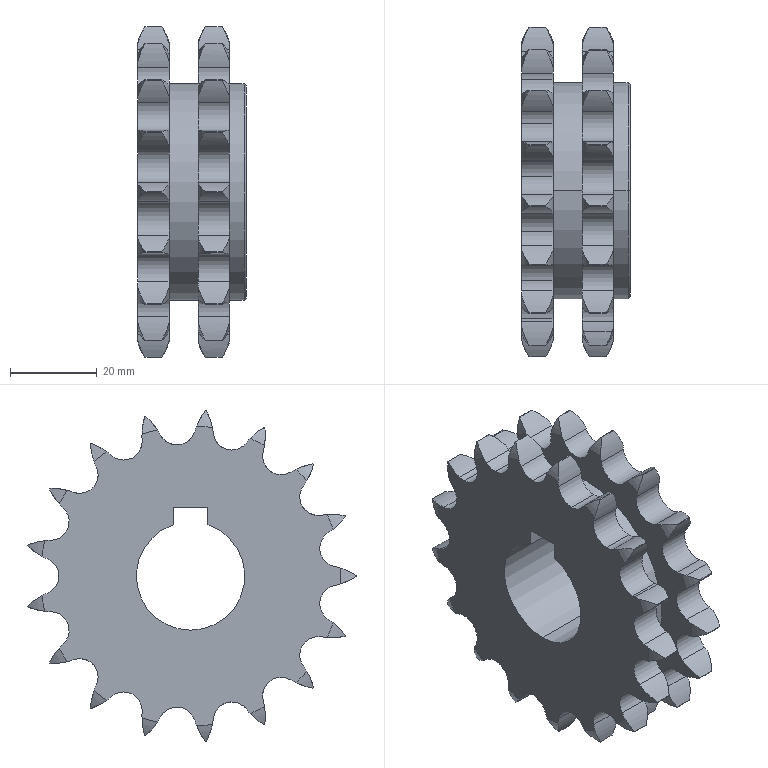Part | SolidWorks | features BaseBody 1 | 1 solid | 236 faces | box 25 x 75.844 x 76.169 mm | volume 56739 mm3 | cylinder 158 | spline 68 | plane 8 | cone 2 | commonest cylinder face diameters 30.636 x72 8.51 x46 76.481 x34 50 x4 25 x2